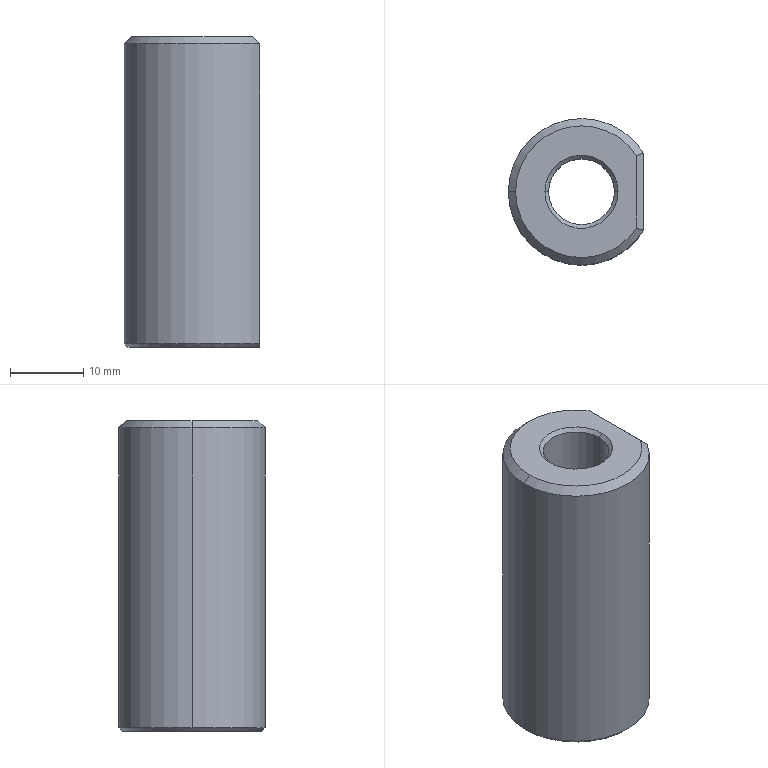Part | STEP file | Limit sleeve | 1 solid | 19 faces | box 18.5 x 20 x 42.5 mm | volume 8069 mm3 | cone 9 | cylinder 6 | plane 4 | commonest cylinder face diameters 9 x2 15 x2 20 x2
STEP:
#1=CARTESIAN_POINT('',(0.,0.,0.));
#2=DIRECTION('',(0.,0.,1.));
#3=DIRECTION('',(1.,0.,0.));
#4=AXIS2_PLACEMENT_3D('',#1,#2,#3);
#5=CARTESIAN_POINT('',(8.5,-5.268,41.5));
#6=VERTEX_POINT('',#5);
#7=CARTESIAN_POINT('',(-10.,0.,41.5));
#8=VERTEX_POINT('',#7);
#9=CARTESIAN_POINT('',(0.,0.,41.5));
#10=DIRECTION('',(0.,0.,-1.));
#11=DIRECTION('',(-1.,0.,0.));
#12=AXIS2_PLACEMENT_3D('',#9,#10,#11);
#13=CIRCLE('',#12,10.);
#14=CARTESIAN_POINT('',(0.,0.,42.5));
#15=DIRECTION('',(0.,0.,-1.));
#16=DIRECTION('',(-1.,0.,0.));
#17=AXIS2_PLACEMENT_3D('',#14,#15,#16);
#18=CYLINDRICAL_SURFACE('',#17,10.);
#19=CARTESIAN_POINT('',(0.,1.));
#20=DIRECTION('',(1.,0.));
#21=VECTOR('',#20,1.);
#22=LINE('',#19,#21);
#23=(GEOMETRIC_REPRESENTATION_CONTEXT(2)PARAMETRIC_REPRESENTATION_CONTEXT()REPRESENTATION_CONTEXT('',''));
#24=DEFINITIONAL_REPRESENTATION('',(#22),#23);
#25=PCURVE('',#18,#24);
#26=CARTESIAN_POINT('',(0.,0.,41.5));
#27=DIRECTION('',(0.,0.,-1.));
#28=DIRECTION('',(-1.,0.,0.));
#29=AXIS2_PLACEMENT_3D('',#26,#27,#28);
#30=CONICAL_SURFACE('',#29,10.,0.7854);
#31=CARTESIAN_POINT('',(0.,0.));
#32=DIRECTION('',(1.,0.));
#33=VECTOR('',#32,1.);
#34=LINE('',#31,#33);
#35=(GEOMETRIC_REPRESENTATION_CONTEXT(2)PARAMETRIC_REPRESENTATION_CONTEXT()REPRESENTATION_CONTEXT('',''));
#36=DEFINITIONAL_REPRESENTATION('',(#34),#35);
#37=PCURVE('',#30,#36);
#38=SURFACE_CURVE('',#13,(#25,#37),.PCURVE_S1.);
#39=EDGE_CURVE('',#6,#8,#38,.T.);
#40=ORIENTED_EDGE('',*,*,#39,.T.);
#41=CARTESIAN_POINT('',(-10.,0.,0.5));
#42=VERTEX_POINT('',#41);
#43=CARTESIAN_POINT('',(-10.,0.,42.5));
#44=DIRECTION('',(0.,0.,-1.));
#45=VECTOR('',#44,1.);
#46=LINE('',#43,#45);
#47=CARTESIAN_POINT('',(6.283,0.));
#48=DIRECTION('',(0.,1.));
#49=VECTOR('',#48,1.);
#50=LINE('',#47,#49);
#51=(GEOMETRIC_REPRESENTATION_CONTEXT(2)PARAMETRIC_REPRESENTATION_CONTEXT()REPRESENTATION_CONTEXT('',''));
#52=DEFINITIONAL_REPRESENTATION('',(#50),#51);
#53=PCURVE('',#18,#52);
#54=CARTESIAN_POINT('',(0.,0.,42.5));
#55=DIRECTION('',(0.,0.,-1.));
#56=DIRECTION('',(-1.,0.,0.));
#57=AXIS2_PLACEMENT_3D('',#54,#55,#56);
#58=CYLINDRICAL_SURFACE('',#57,10.);
#59=CARTESIAN_POINT('',(0.,0.));
#60=DIRECTION('',(0.,1.));
#61=VECTOR('',#60,1.);
#62=LINE('',#59,#61);
#63=(GEOMETRIC_REPRESENTATION_CONTEXT(2)PARAMETRIC_REPRESENTATION_CONTEXT()REPRESENTATION_CONTEXT('',''));
#64=DEFINITIONAL_REPRESENTATION('',(#62),#63);
#65=PCURVE('',#58,#64);
#66=SURFACE_CURVE('',#46,(#53,#65),.PCURVE_S1.);
#67=EDGE_CURVE('',#8,#42,#66,.T.);
#68=ORIENTED_EDGE('',*,*,#67,.T.);
#69=CARTESIAN_POINT('',(8.5,-5.268,0.5));
#70=VERTEX_POINT('',#69);
#71=CARTESIAN_POINT('',(0.,0.,0.5));
#72=DIRECTION('',(0.,0.,1.));
#73=DIRECTION('',(-1.,0.,0.));
#74=AXIS2_PLACEMENT_3D('',#71,#72,#73);
#75=CIRCLE('',#74,10.);
#76=CARTESIAN_POINT('',(6.283,42.));
#77=DIRECTION('',(-1.,0.));
#78=VECTOR('',#77,1.);
#79=LINE('',#76,#78);
#80=(GEOMETRIC_REPRESENTATION_CONTEXT(2)PARAMETRIC_REPRESENTATION_CONTEXT()REPRESENTATION_CONTEXT('',''));
#81=DEFINITIONAL_REPRESENTATION('',(#79),#80);
#82=PCURVE('',#18,#81);
#83=CARTESIAN_POINT('',(0.,0.,0.5));
#84=DIRECTION('',(0.,0.,1.));
#85=DIRECTION('',(1.,0.,0.));
#86=AXIS2_PLACEMENT_3D('',#83,#84,#85);
#87=CONICAL_SURFACE('',#86,10.,0.7854);
#88=CARTESIAN_POINT('',(3.142,0.));
#89=DIRECTION('',(1.,0.));
#90=VECTOR('',#89,1.);
#91=LINE('',#88,#90);
#92=(GEOMETRIC_REPRESENTATION_CONTEXT(2)PARAMETRIC_REPRESENTATION_CONTEXT()REPRESENTATION_CONTEXT('',''));
#93=DEFINITIONAL_REPRESENTATION('',(#91),#92);
#94=PCURVE('',#87,#93);
#95=SURFACE_CURVE('',#75,(#82,#94),.PCURVE_S1.);
#96=EDGE_CURVE('',#42,#70,#95,.T.);
#97=ORIENTED_EDGE('',*,*,#96,.T.);
#98=CARTESIAN_POINT('',(8.5,-5.268,42.5));
#99=DIRECTION('',(0.,0.,1.));
#100=VECTOR('',#99,1.);
#101=LINE('',#98,#100);
#102=CARTESIAN_POINT('',(3.696,0.));
#103=DIRECTION('',(0.,-1.));
#104=VECTOR('',#103,1.);
#105=LINE('',#102,#104);
#106=(GEOMETRIC_REPRESENTATION_CONTEXT(2)PARAMETRIC_REPRESENTATION_CONTEXT()REPRESENTATION_CONTEXT('',''));
#107=DEFINITIONAL_REPRESENTATION('',(#105),#106);
#108=PCURVE('',#18,#107);
#109=CARTESIAN_POINT('',(8.5,5.268,42.5));
#110=DIRECTION('',(-1.,0.,0.));
#111=DIRECTION('',(0.,0.,1.));
#112=AXIS2_PLACEMENT_3D('',#109,#110,#111);
#113=PLANE('',#112);
#114=CARTESIAN_POINT('',(0.,-10.536));
#115=DIRECTION('',(1.,0.));
#116=VECTOR('',#115,1.);
#117=LINE('',#114,#116);
#118=(GEOMETRIC_REPRESENTATION_CONTEXT(2)PARAMETRIC_REPRESENTATION_CONTEXT()REPRESENTATION_CONTEXT('',''));
#119=DEFINITIONAL_REPRESENTATION('',(#117),#118);
#120=PCURVE('',#113,#119);
#121=SURFACE_CURVE('',#101,(#108,#120),.PCURVE_S1.);
#122=EDGE_CURVE('',#70,#6,#121,.T.);
#123=ORIENTED_EDGE('',*,*,#122,.T.);
#124=EDGE_LOOP('',(#40,#68,#97,#123));
#125=FACE_BOUND('',#124,.T.);
#126=ADVANCED_FACE('',(#125),#18,.T.);
#127=CARTESIAN_POINT('',(7.5,-4.975,42.5));
#128=VERTEX_POINT('',#127);
#129=CARTESIAN_POINT('',(-9.,0.,42.5));
#130=VERTEX_POINT('',#129);
#131=CARTESIAN_POINT('',(0.,0.,42.5));
#132=DIRECTION('',(0.,0.,-1.));
#133=DIRECTION('',(-1.,0.,0.));
#134=AXIS2_PLACEMENT_3D('',#131,#132,#133);
#135=CIRCLE('',#134,9.);
#136=CARTESIAN_POINT('',(0.,-1.));
#137=DIRECTION('',(1.,0.));
#138=VECTOR('',#137,1.);
#139=LINE('',#136,#138);
#140=(GEOMETRIC_REPRESENTATION_CONTEXT(2)PARAMETRIC_REPRESENTATION_CONTEXT()REPRESENTATION_CONTEXT('',''));
#141=DEFINITIONAL_REPRESENTATION('',(#139),#140);
#142=PCURVE('',#30,#141);
#143=CARTESIAN_POINT('',(0.,0.,42.5));
#144=DIRECTION('',(0.,0.,1.));
#145=DIRECTION('',(1.,0.,0.));
#146=AXIS2_PLACEMENT_3D('',#143,#144,#145);
#147=PLANE('',#146);
#148=CARTESIAN_POINT('',(-9.,0.));
#149=CARTESIAN_POINT('',(-9.,15.588));
#150=CARTESIAN_POINT('',(4.5,7.794));
#151=CARTESIAN_POINT('',(18.,0.));
#152=CARTESIAN_POINT('',(4.5,-7.794));
#153=CARTESIAN_POINT('',(-9.,-15.588));
#154=CARTESIAN_POINT('',(-9.,0.));
#155=(BOUNDED_CURVE()B_SPLINE_CURVE(2,(#148,#149,#150,#151,#152,#153,#154),.UNSPECIFIED.,.T.,.F.)B_SPLINE_CURVE_WITH_KNOTS((1,2,2,2,2,1),(-2.094,0.,2.094,4.189,6.283,8.378),.UNSPECIFIED.)CURVE()GEOMETRIC_REPRESENTATION_ITEM()RATIONAL_B_SPLINE_CURVE((1.,0.5,1.,0.5,1.,0.5,1.))REPRESENTATION_ITEM(''));
#156=(GEOMETRIC_REPRESENTATION_CONTEXT(2)PARAMETRIC_REPRESENTATION_CONTEXT()REPRESENTATION_CONTEXT('',''));
#157=DEFINITIONAL_REPRESENTATION('',(#155),#156);
#158=PCURVE('',#147,#157);
#159=SURFACE_CURVE('',#135,(#142,#158),.PCURVE_S1.);
#160=EDGE_CURVE('',#128,#130,#159,.T.);
#161=ORIENTED_EDGE('',*,*,#160,.T.);
#162=CARTESIAN_POINT('',(-10.,0.,41.5));
#163=DIRECTION('',(-0.7071,0.,-0.7071));
#164=VECTOR('',#163,1.);
#165=LINE('',#162,#164);
#166=CARTESIAN_POINT('',(6.283,0.));
#167=DIRECTION('',(0.,1.));
#168=VECTOR('',#167,1.);
#169=LINE('',#166,#168);
#170=(GEOMETRIC_REPRESENTATION_CONTEXT(2)PARAMETRIC_REPRESENTATION_CONTEXT()REPRESENTATION_CONTEXT('',''));
#171=DEFINITIONAL_REPRESENTATION('',(#169),#170);
#172=PCURVE('',#30,#171);
#173=CARTESIAN_POINT('',(0.,0.,41.5));
#174=DIRECTION('',(0.,0.,-1.));
#175=DIRECTION('',(-1.,0.,0.));
#176=AXIS2_PLACEMENT_3D('',#173,#174,#175);
#177=CONICAL_SURFACE('',#176,10.,0.7854);
#178=CARTESIAN_POINT('',(0.,0.));
#179=DIRECTION('',(0.,1.));
#180=VECTOR('',#179,1.);
#181=LINE('',#178,#180);
#182=(GEOMETRIC_REPRESENTATION_CONTEXT(2)PARAMETRIC_REPRESENTATION_CONTEXT()REPRESENTATION_CONTEXT('',''));
#183=DEFINITIONAL_REPRESENTATION('',(#181),#182);
#184=PCURVE('',#177,#183);
#185=SURFACE_CURVE('',#165,(#172,#184),.PCURVE_S1.);
#186=EDGE_CURVE('',#130,#8,#185,.T.);
#187=ORIENTED_EDGE('',*,*,#186,.T.);
#188=ORIENTED_EDGE('',*,*,#39,.F.);
#189=CARTESIAN_POINT('',(8.5,-5.268,41.5));
#190=CARTESIAN_POINT('',(8.152,-5.169,41.848));
#191=CARTESIAN_POINT('',(7.818,-5.071,42.182));
#192=CARTESIAN_POINT('',(7.5,-4.975,42.5));
#193=B_SPLINE_CURVE_WITH_KNOTS('',3,(#189,#190,#191,#192),.UNSPECIFIED.,.F.,.F.,(4,4),(0.,1.),.PIECEWISE_BEZIER_KNOTS.);
#194=CARTESIAN_POINT('',(3.696,0.));
#195=CARTESIAN_POINT('',(3.697,-0.01584));
#196=CARTESIAN_POINT('',(3.698,-0.04744));
#197=CARTESIAN_POINT('',(3.699,-0.09467));
#198=CARTESIAN_POINT('',(3.7,-0.1417));
#199=CARTESIAN_POINT('',(3.702,-0.1886));
#200=CARTESIAN_POINT('',(3.703,-0.2352));
#201=CARTESIAN_POINT('',(3.705,-0.2817));
#202=CARTESIAN_POINT('',(3.706,-0.328));
#203=CARTESIAN_POINT('',(3.707,-0.3741));
#204=CARTESIAN_POINT('',(3.709,-0.42));
#205=CARTESIAN_POINT('',(3.71,-0.4658));
#206=CARTESIAN_POINT('',(3.712,-0.5113));
#207=CARTESIAN_POINT('',(3.713,-0.5567));
#208=CARTESIAN_POINT('',(3.714,-0.6019));
#209=CARTESIAN_POINT('',(3.716,-0.6468));
#210=CARTESIAN_POINT('',(3.717,-0.6916));
#211=CARTESIAN_POINT('',(3.719,-0.7363));
#212=CARTESIAN_POINT('',(3.72,-0.7807));
#213=CARTESIAN_POINT('',(3.721,-0.8249));
#214=CARTESIAN_POINT('',(3.723,-0.869));
#215=CARTESIAN_POINT('',(3.724,-0.9129));
#216=CARTESIAN_POINT('',(3.726,-0.9565));
#217=CARTESIAN_POINT('',(3.727,-0.9855));
#218=CARTESIAN_POINT('',(3.727,-1.));
#219=B_SPLINE_CURVE_WITH_KNOTS('',3,(#194,#195,#196,#197,#198,#199,#200,#201,#202,#203,#204,#205,#206,#207,#208,#209,#210,#211,#212,#213,#214,#215,#216,#217,#218),.UNSPECIFIED.,.F.,.F.,(4,1,1,1,1,1,1,1,1,1,1,1,1,1,1,1,1,1,1,1,1,1,4),(0.,0.04545,0.09091,0.1364,0.1818,0.2273,0.2727,0.3182,0.3636,0.4091,0.4545,0.5,0.5455,0.5909,0.6364,0.6818,0.7273,0.7727,0.8182,0.8636,0.9091,0.9545,1.),.QUASI_UNIFORM_KNOTS.);
#220=(GEOMETRIC_REPRESENTATION_CONTEXT(2)PARAMETRIC_REPRESENTATION_CONTEXT()REPRESENTATION_CONTEXT('',''));
#221=DEFINITIONAL_REPRESENTATION('',(#219),#220);
#222=PCURVE('',#30,#221);
#223=CARTESIAN_POINT('',(7.5,0.,42.5));
#224=DIRECTION('',(0.7071,0.,0.7071));
#225=DIRECTION('',(0.7071,0.,-0.7071));
#226=AXIS2_PLACEMENT_3D('',#223,#224,#225);
#227=PLANE('',#226);
#228=CARTESIAN_POINT('',(1.414,-5.268));
#229=CARTESIAN_POINT('',(0.9215,-5.169));
#230=CARTESIAN_POINT('',(0.4501,-5.071));
#231=CARTESIAN_POINT('',(0.,-4.975));
#232=B_SPLINE_CURVE_WITH_KNOTS('',3,(#228,#229,#230,#231),.UNSPECIFIED.,.F.,.F.,(4,4),(0.,1.),.PIECEWISE_BEZIER_KNOTS.);
#233=(GEOMETRIC_REPRESENTATION_CONTEXT(2)PARAMETRIC_REPRESENTATION_CONTEXT()REPRESENTATION_CONTEXT('',''));
#234=DEFINITIONAL_REPRESENTATION('',(#232),#233);
#235=PCURVE('',#227,#234);
#236=SURFACE_CURVE('',#193,(#222,#235),.PCURVE_S1.);
#237=EDGE_CURVE('',#6,#128,#236,.T.);
#238=ORIENTED_EDGE('',*,*,#237,.T.);
#239=EDGE_LOOP('',(#161,#187,#188,#238));
#240=FACE_BOUND('',#239,.T.);
#241=ADVANCED_FACE('',(#240),#30,.T.);
#242=CARTESIAN_POINT('',(-7.5,0.,0.5));
#243=VERTEX_POINT('',#242);
#244=CARTESIAN_POINT('',(-8.,0.,0.));
#245=VERTEX_POINT('',#244);
#246=CARTESIAN_POINT('',(-8.,0.,0.));
#247=DIRECTION('',(-0.7071,0.,-0.7071));
#248=VECTOR('',#247,1.);
#249=LINE('',#246,#248);
#250=CARTESIAN_POINT('',(0.,0.,0.));
#251=DIRECTION('',(0.,0.,-1.));
#252=DIRECTION('',(-1.,0.,0.));
#253=AXIS2_PLACEMENT_3D('',#250,#251,#252);
#254=CONICAL_SURFACE('',#253,8.,0.7854);
#255=CARTESIAN_POINT('',(6.283,0.));
#256=DIRECTION('',(0.,1.));
#257=VECTOR('',#256,1.);
#258=LINE('',#255,#257);
#259=(GEOMETRIC_REPRESENTATION_CONTEXT(2)PARAMETRIC_REPRESENTATION_CONTEXT()REPRESENTATION_CONTEXT('',''));
#260=DEFINITIONAL_REPRESENTATION('',(#258),#259);
#261=PCURVE('',#254,#260);
#262=CARTESIAN_POINT('',(0.,0.,0.));
#263=DIRECTION('',(0.,0.,-1.));
#264=DIRECTION('',(-1.,0.,0.));
#265=AXIS2_PLACEMENT_3D('',#262,#263,#264);
#266=CONICAL_SURFACE('',#265,8.,0.7854);
#267=CARTESIAN_POINT('',(0.,0.));
#268=DIRECTION('',(0.,1.));
#269=VECTOR('',#268,1.);
#270=LINE('',#267,#269);
#271=(GEOMETRIC_REPRESENTATION_CONTEXT(2)PARAMETRIC_REPRESENTATION_CONTEXT()REPRESENTATION_CONTEXT('',''));
#272=DEFINITIONAL_REPRESENTATION('',(#270),#271);
#273=PCURVE('',#266,#272);
#274=SURFACE_CURVE('',#249,(#261,#273),.PCURVE_S1.);
#275=EDGE_CURVE('',#243,#245,#274,.T.);
#276=ORIENTED_EDGE('',*,*,#275,.T.);
#277=CARTESIAN_POINT('',(8.,0.,0.));
#278=VERTEX_POINT('',#277);
#279=CARTESIAN_POINT('',(0.,0.,0.));
#280=DIRECTION('',(0.,0.,-1.));
#281=DIRECTION('',(-1.,0.,0.));
#282=AXIS2_PLACEMENT_3D('',#279,#280,#281);
#283=CIRCLE('',#282,8.);
#284=CARTESIAN_POINT('',(0.,0.));
#285=DIRECTION('',(1.,0.));
#286=VECTOR('',#285,1.);
#287=LINE('',#284,#286);
#288=(GEOMETRIC_REPRESENTATION_CONTEXT(2)PARAMETRIC_REPRESENTATION_CONTEXT()REPRESENTATION_CONTEXT('',''));
#289=DEFINITIONAL_REPRESENTATION('',(#287),#288);
#290=PCURVE('',#254,#289);
#291=CARTESIAN_POINT('',(0.,0.,0.));
#292=DIRECTION('',(0.,0.,1.));
#293=DIRECTION('',(1.,0.,0.));
#294=AXIS2_PLACEMENT_3D('',#291,#292,#293);
#295=PLANE('',#294);
#296=CARTESIAN_POINT('',(-8.,0.));
#297=CARTESIAN_POINT('',(-8.,13.856));
#298=CARTESIAN_POINT('',(4.,6.928));
#299=CARTESIAN_POINT('',(16.,0.));
#300=CARTESIAN_POINT('',(4.,-6.928));
#301=CARTESIAN_POINT('',(-8.,-13.856));
#302=CARTESIAN_POINT('',(-8.,0.));
#303=(BOUNDED_CURVE()B_SPLINE_CURVE(2,(#296,#297,#298,#299,#300,#301,#302),.UNSPECIFIED.,.T.,.F.)B_SPLINE_CURVE_WITH_KNOTS((1,2,2,2,2,1),(-2.094,0.,2.094,4.189,6.283,8.378),.UNSPECIFIED.)CURVE()GEOMETRIC_REPRESENTATION_ITEM()RATIONAL_B_SPLINE_CURVE((1.,0.5,1.,0.5,1.,0.5,1.))REPRESENTATION_ITEM(''));
#304=(GEOMETRIC_REPRESENTATION_CONTEXT(2)PARAMETRIC_REPRESENTATION_CONTEXT()REPRESENTATION_CONTEXT('',''));
#305=DEFINITIONAL_REPRESENTATION('',(#303),#304);
#306=PCURVE('',#295,#305);
#307=SURFACE_CURVE('',#283,(#290,#306),.PCURVE_S1.);
#308=EDGE_CURVE('',#278,#245,#307,.T.);
#309=ORIENTED_EDGE('',*,*,#308,.F.);
#310=CARTESIAN_POINT('',(7.5,0.,0.5));
#311=VERTEX_POINT('',#310);
#312=CARTESIAN_POINT('',(8.,0.,0.));
#313=DIRECTION('',(0.7071,0.,-0.7071));
#314=VECTOR('',#313,1.);
#315=LINE('',#312,#314);
#316=CARTESIAN_POINT('',(3.142,0.));
#317=DIRECTION('',(0.,1.));
#318=VECTOR('',#317,1.);
#319=LINE('',#316,#318);
#320=(GEOMETRIC_REPRESENTATION_CONTEXT(2)PARAMETRIC_REPRESENTATION_CONTEXT()REPRESENTATION_CONTEXT('',''));
#321=DEFINITIONAL_REPRESENTATION('',(#319),#320);
#322=PCURVE('',#254,#321);
#323=CARTESIAN_POINT('',(3.142,0.));
#324=DIRECTION('',(0.,1.));
#325=VECTOR('',#324,1.);
#326=LINE('',#323,#325);
#327=(GEOMETRIC_REPRESENTATION_CONTEXT(2)PARAMETRIC_REPRESENTATION_CONTEXT()REPRESENTATION_CONTEXT('',''));
#328=DEFINITIONAL_REPRESENTATION('',(#326),#327);
#329=PCURVE('',#266,#328);
#330=SURFACE_CURVE('',#315,(#322,#329),.PCURVE_S1.);
#331=EDGE_CURVE('',#311,#278,#330,.T.);
#332=ORIENTED_EDGE('',*,*,#331,.F.);
#333=CARTESIAN_POINT('',(0.,0.,0.5));
#334=DIRECTION('',(0.,0.,-1.));
#335=DIRECTION('',(-1.,0.,0.));
#336=AXIS2_PLACEMENT_3D('',#333,#334,#335);
#337=CIRCLE('',#336,7.5);
#338=CARTESIAN_POINT('',(0.,-0.5));
#339=DIRECTION('',(1.,0.));
#340=VECTOR('',#339,1.);
#341=LINE('',#338,#340);
#342=(GEOMETRIC_REPRESENTATION_CONTEXT(2)PARAMETRIC_REPRESENTATION_CONTEXT()REPRESENTATION_CONTEXT('',''));
#343=DEFINITIONAL_REPRESENTATION('',(#341),#342);
#344=PCURVE('',#254,#343);
#345=CARTESIAN_POINT('',(0.,0.,17.));
#346=DIRECTION('',(0.,0.,-1.));
#347=DIRECTION('',(-1.,0.,0.));
#348=AXIS2_PLACEMENT_3D('',#345,#346,#347);
#349=CYLINDRICAL_SURFACE('',#348,7.5);
#350=CARTESIAN_POINT('',(0.,16.5));
#351=DIRECTION('',(1.,0.));
#352=VECTOR('',#351,1.);
#353=LINE('',#350,#352);
#354=(GEOMETRIC_REPRESENTATION_CONTEXT(2)PARAMETRIC_REPRESENTATION_CONTEXT()REPRESENTATION_CONTEXT('',''));
#355=DEFINITIONAL_REPRESENTATION('',(#353),#354);
#356=PCURVE('',#349,#355);
#357=SURFACE_CURVE('',#337,(#344,#356),.PCURVE_S1.);
#358=EDGE_CURVE('',#311,#243,#357,.T.);
#359=ORIENTED_EDGE('',*,*,#358,.T.);
#360=EDGE_LOOP('',(#276,#309,#332,#359));
#361=FACE_BOUND('',#360,.F.);
#362=ADVANCED_FACE('',(#361),#254,.F.);
#363=CARTESIAN_POINT('',(4.5,0.,42.));
#364=VERTEX_POINT('',#363);
#365=CARTESIAN_POINT('',(5.,0.,42.5));
#366=VERTEX_POINT('',#365);
#367=CARTESIAN_POINT('',(5.,0.,42.5));
#368=DIRECTION('',(0.7071,0.,0.7071));
#369=VECTOR('',#368,1.);
#370=LINE('',#367,#369);
#371=CARTESIAN_POINT('',(0.,0.,42.5));
#372=DIRECTION('',(0.,0.,1.));
#373=DIRECTION('',(1.,0.,0.));
#374=AXIS2_PLACEMENT_3D('',#371,#372,#373);
#375=CONICAL_SURFACE('',#374,5.,0.7854);
#376=CARTESIAN_POINT('',(6.283,0.));
#377=DIRECTION('',(0.,1.));
#378=VECTOR('',#377,1.);
#379=LINE('',#376,#378);
#380=(GEOMETRIC_REPRESENTATION_CONTEXT(2)PARAMETRIC_REPRESENTATION_CONTEXT()REPRESENTATION_CONTEXT('',''));
#381=DEFINITIONAL_REPRESENTATION('',(#379),#380);
#382=PCURVE('',#375,#381);
#383=CARTESIAN_POINT('',(0.,0.,42.5));
#384=DIRECTION('',(0.,0.,1.));
#385=DIRECTION('',(1.,0.,0.));
#386=AXIS2_PLACEMENT_3D('',#383,#384,#385);
#387=CONICAL_SURFACE('',#386,5.,0.7854);
#388=CARTESIAN_POINT('',(0.,0.));
#389=DIRECTION('',(0.,1.));
#390=VECTOR('',#389,1.);
#391=LINE('',#388,#390);
#392=(GEOMETRIC_REPRESENTATION_CONTEXT(2)PARAMETRIC_REPRESENTATION_CONTEXT()REPRESENTATION_CONTEXT('',''));
#393=DEFINITIONAL_REPRESENTATION('',(#391),#392);
#394=PCURVE('',#387,#393);
#395=SURFACE_CURVE('',#370,(#382,#394),.PCURVE_S1.);
#396=EDGE_CURVE('',#364,#366,#395,.T.);
#397=ORIENTED_EDGE('',*,*,#396,.T.);
#398=CARTESIAN_POINT('',(-5.,0.,42.5));
#399=VERTEX_POINT('',#398);
#400=CARTESIAN_POINT('',(0.,0.,42.5));
#401=DIRECTION('',(0.,0.,-1.));
#402=DIRECTION('',(1.,0.,0.));
#403=AXIS2_PLACEMENT_3D('',#400,#401,#402);
#404=CIRCLE('',#403,5.);
#405=CARTESIAN_POINT('',(6.283,0.));
#406=DIRECTION('',(-1.,0.));
#407=VECTOR('',#406,1.);
#408=LINE('',#405,#407);
#409=(GEOMETRIC_REPRESENTATION_CONTEXT(2)PARAMETRIC_REPRESENTATION_CONTEXT()REPRESENTATION_CONTEXT('',''));
#410=DEFINITIONAL_REPRESENTATION('',(#408),#409);
#411=PCURVE('',#375,#410);
#412=CARTESIAN_POINT('',(5.,0.));
#413=CARTESIAN_POINT('',(5.,-8.66));
#414=CARTESIAN_POINT('',(-2.5,-4.33));
#415=CARTESIAN_POINT('',(-10.,0.));
#416=CARTESIAN_POINT('',(-2.5,4.33));
#417=CARTESIAN_POINT('',(5.,8.66));
#418=CARTESIAN_POINT('',(5.,0.));
#419=(BOUNDED_CURVE()B_SPLINE_CURVE(2,(#412,#413,#414,#415,#416,#417,#418),.UNSPECIFIED.,.T.,.F.)B_SPLINE_CURVE_WITH_KNOTS((1,2,2,2,2,1),(-2.094,0.,2.094,4.189,6.283,8.378),.UNSPECIFIED.)CURVE()GEOMETRIC_REPRESENTATION_ITEM()RATIONAL_B_SPLINE_CURVE((1.,0.5,1.,0.5,1.,0.5,1.))REPRESENTATION_ITEM(''));
#420=(GEOMETRIC_REPRESENTATION_CONTEXT(2)PARAMETRIC_REPRESENTATION_CONTEXT()REPRESENTATION_CONTEXT('',''));
#421=DEFINITIONAL_REPRESENTATION('',(#419),#420);
#422=PCURVE('',#147,#421);
#423=SURFACE_CURVE('',#404,(#411,#422),.PCURVE_S1.);
#424=EDGE_CURVE('',#366,#399,#423,.T.);
#425=ORIENTED_EDGE('',*,*,#424,.T.);
#426=CARTESIAN_POINT('',(-4.5,0.,42.));
#427=VERTEX_POINT('',#426);
#428=CARTESIAN_POINT('',(-5.,0.,42.5));
#429=DIRECTION('',(-0.7071,0.,0.7071));
#430=VECTOR('',#429,1.);
#431=LINE('',#428,#430);
#432=CARTESIAN_POINT('',(3.142,0.));
#433=DIRECTION('',(0.,1.));
#434=VECTOR('',#433,1.);
#435=LINE('',#432,#434);
#436=(GEOMETRIC_REPRESENTATION_CONTEXT(2)PARAMETRIC_REPRESENTATION_CONTEXT()REPRESENTATION_CONTEXT('',''));
#437=DEFINITIONAL_REPRESENTATION('',(#435),#436);
#438=PCURVE('',#375,#437);
#439=CARTESIAN_POINT('',(3.142,0.));
#440=DIRECTION('',(0.,1.));
#441=VECTOR('',#440,1.);
#442=LINE('',#439,#441);
#443=(GEOMETRIC_REPRESENTATION_CONTEXT(2)PARAMETRIC_REPRESENTATION_CONTEXT()REPRESENTATION_CONTEXT('',''));
#444=DEFINITIONAL_REPRESENTATION('',(#442),#443);
#445=PCURVE('',#387,#444);
#446=SURFACE_CURVE('',#431,(#438,#445),.PCURVE_S1.);
#447=EDGE_CURVE('',#427,#399,#446,.T.);
#448=ORIENTED_EDGE('',*,*,#447,.F.);
#449=CARTESIAN_POINT('',(0.,0.,42.));
#450=DIRECTION('',(0.,0.,1.));
#451=DIRECTION('',(1.,0.,0.));
#452=AXIS2_PLACEMENT_3D('',#449,#450,#451);
#453=CIRCLE('',#452,4.5);
#454=CARTESIAN_POINT('',(0.,-0.5));
#455=DIRECTION('',(1.,0.));
#456=VECTOR('',#455,1.);
#457=LINE('',#454,#456);
#458=(GEOMETRIC_REPRESENTATION_CONTEXT(2)PARAMETRIC_REPRESENTATION_CONTEXT()REPRESENTATION_CONTEXT('',''));
#459=DEFINITIONAL_REPRESENTATION('',(#457),#458);
#460=PCURVE('',#375,#459);
#461=CARTESIAN_POINT('',(0.,0.,0.));
#462=DIRECTION('',(0.,0.,1.));
#463=DIRECTION('',(1.,0.,0.));
#464=AXIS2_PLACEMENT_3D('',#461,#462,#463);
#465=CYLINDRICAL_SURFACE('',#464,4.5);
#466=CARTESIAN_POINT('',(0.,42.));
#467=DIRECTION('',(1.,0.));
#468=VECTOR('',#467,1.);
#469=LINE('',#466,#468);
#470=(GEOMETRIC_REPRESENTATION_CONTEXT(2)PARAMETRIC_REPRESENTATION_CONTEXT()REPRESENTATION_CONTEXT('',''));
#471=DEFINITIONAL_REPRESENTATION('',(#469),#470);
#472=PCURVE('',#465,#471);
#473=SURFACE_CURVE('',#453,(#460,#472),.PCURVE_S1.);
#474=EDGE_CURVE('',#427,#364,#473,.T.);
#475=ORIENTED_EDGE('',*,*,#474,.T.);
#476=EDGE_LOOP('',(#397,#425,#448,#475));
#477=FACE_BOUND('',#476,.F.);
#478=ADVANCED_FACE('',(#477),#375,.F.);
#479=CARTESIAN_POINT('',(-7.5,0.,17.));
#480=VERTEX_POINT('',#479);
#481=CARTESIAN_POINT('',(-7.5,0.,17.));
#482=DIRECTION('',(0.,0.,-1.));
#483=VECTOR('',#482,1.);
#484=LINE('',#481,#483);
#485=CARTESIAN_POINT('',(6.283,0.));
#486=DIRECTION('',(0.,1.));
#487=VECTOR('',#486,1.);
#488=LINE('',#485,#487);
#489=(GEOMETRIC_REPRESENTATION_CONTEXT(2)PARAMETRIC_REPRESENTATION_CONTEXT()REPRESENTATION_CONTEXT('',''));
#490=DEFINITIONAL_REPRESENTATION('',(#488),#489);
#491=PCURVE('',#349,#490);
#492=CARTESIAN_POINT('',(0.,0.,17.));
#493=DIRECTION('',(0.,0.,-1.));
#494=DIRECTION('',(-1.,0.,0.));
#495=AXIS2_PLACEMENT_3D('',#492,#493,#494);
#496=CYLINDRICAL_SURFACE('',#495,7.5);
#497=CARTESIAN_POINT('',(0.,0.));
#498=DIRECTION('',(0.,1.));
#499=VECTOR('',#498,1.);
#500=LINE('',#497,#499);
#501=(GEOMETRIC_REPRESENTATION_CONTEXT(2)PARAMETRIC_REPRESENTATION_CONTEXT()REPRESENTATION_CONTEXT('',''));
#502=DEFINITIONAL_REPRESENTATION('',(#500),#501);
#503=PCURVE('',#496,#502);
#504=SURFACE_CURVE('',#484,(#491,#503),.PCURVE_S1.);
#505=EDGE_CURVE('',#480,#243,#504,.T.);
#506=ORIENTED_EDGE('',*,*,#505,.T.);
#507=ORIENTED_EDGE('',*,*,#358,.F.);
#508=CARTESIAN_POINT('',(7.5,0.,17.));
#509=VERTEX_POINT('',#508);
#510=CARTESIAN_POINT('',(7.5,0.,17.));
#511=DIRECTION('',(0.,0.,-1.));
#512=VECTOR('',#511,1.);
#513=LINE('',#510,#512);
#514=CARTESIAN_POINT('',(3.142,0.));
#515=DIRECTION('',(0.,1.));
#516=VECTOR('',#515,1.);
#517=LINE('',#514,#516);
#518=(GEOMETRIC_REPRESENTATION_CONTEXT(2)PARAMETRIC_REPRESENTATION_CONTEXT()REPRESENTATION_CONTEXT('',''));
#519=DEFINITIONAL_REPRESENTATION('',(#517),#518);
#520=PCURVE('',#349,#519);
#521=CARTESIAN_POINT('',(3.142,0.));
#522=DIRECTION('',(0.,1.));
#523=VECTOR('',#522,1.);
#524=LINE('',#521,#523);
#525=(GEOMETRIC_REPRESENTATION_CONTEXT(2)PARAMETRIC_REPRESENTATION_CONTEXT()REPRESENTATION_CONTEXT('',''));
#526=DEFINITIONAL_REPRESENTATION('',(#524),#525);
#527=PCURVE('',#496,#526);
#528=SURFACE_CURVE('',#513,(#520,#527),.PCURVE_S1.);
#529=EDGE_CURVE('',#509,#311,#528,.T.);
#530=ORIENTED_EDGE('',*,*,#529,.F.);
#531=CARTESIAN_POINT('',(0.,0.,17.));
#532=DIRECTION('',(0.,0.,-1.));
#533=DIRECTION('',(-1.,0.,0.));
#534=AXIS2_PLACEMENT_3D('',#531,#532,#533);
#535=CIRCLE('',#534,7.5);
#536=CARTESIAN_POINT('',(0.,0.));
#537=DIRECTION('',(1.,0.));
#538=VECTOR('',#537,1.);
#539=LINE('',#536,#538);
#540=(GEOMETRIC_REPRESENTATION_CONTEXT(2)PARAMETRIC_REPRESENTATION_CONTEXT()REPRESENTATION_CONTEXT('',''));
#541=DEFINITIONAL_REPRESENTATION('',(#539),#540);
#542=PCURVE('',#349,#541);
#543=CARTESIAN_POINT('',(0.,0.,17.));
#544=DIRECTION('',(0.,0.,-1.));
#545=DIRECTION('',(-1.,0.,0.));
#546=AXIS2_PLACEMENT_3D('',#543,#544,#545);
#547=CONICAL_SURFACE('',#546,7.5,0.7854);
#548=CARTESIAN_POINT('',(0.,0.));
#549=DIRECTION('',(1.,0.));
#550=VECTOR('',#549,1.);
#551=LINE('',#548,#550);
#552=(GEOMETRIC_REPRESENTATION_CONTEXT(2)PARAMETRIC_REPRESENTATION_CONTEXT()REPRESENTATION_CONTEXT('',''));
#553=DEFINITIONAL_REPRESENTATION('',(#551),#552);
#554=PCURVE('',#547,#553);
#555=SURFACE_CURVE('',#535,(#542,#554),.PCURVE_S1.);
#556=EDGE_CURVE('',#509,#480,#555,.T.);
#557=ORIENTED_EDGE('',*,*,#556,.T.);
#558=EDGE_LOOP('',(#506,#507,#530,#557));
#559=FACE_BOUND('',#558,.F.);
#560=ADVANCED_FACE('',(#559),#349,.F.);
#561=CARTESIAN_POINT('',(4.5,0.,20.));
#562=VERTEX_POINT('',#561);
#563=CARTESIAN_POINT('',(4.5,0.,0.));
#564=DIRECTION('',(0.,0.,1.));
#565=VECTOR('',#564,1.);
#566=LINE('',#563,#565);
#567=CARTESIAN_POINT('',(6.283,0.));
#568=DIRECTION('',(0.,1.));
#569=VECTOR('',#568,1.);
#570=LINE('',#567,#569);
#571=(GEOMETRIC_REPRESENTATION_CONTEXT(2)PARAMETRIC_REPRESENTATION_CONTEXT()REPRESENTATION_CONTEXT('',''));
#572=DEFINITIONAL_REPRESENTATION('',(#570),#571);
#573=PCURVE('',#465,#572);
#574=CARTESIAN_POINT('',(0.,0.,0.));
#575=DIRECTION('',(0.,0.,1.));
#576=DIRECTION('',(1.,0.,0.));
#577=AXIS2_PLACEMENT_3D('',#574,#575,#576);
#578=CYLINDRICAL_SURFACE('',#577,4.5);
#579=CARTESIAN_POINT('',(0.,0.));
#580=DIRECTION('',(0.,1.));
#581=VECTOR('',#580,1.);
#582=LINE('',#579,#581);
#583=(GEOMETRIC_REPRESENTATION_CONTEXT(2)PARAMETRIC_REPRESENTATION_CONTEXT()REPRESENTATION_CONTEXT('',''));
#584=DEFINITIONAL_REPRESENTATION('',(#582),#583);
#585=PCURVE('',#578,#584);
#586=SURFACE_CURVE('',#566,(#573,#585),.PCURVE_S1.);
#587=EDGE_CURVE('',#562,#364,#586,.T.);
#588=ORIENTED_EDGE('',*,*,#587,.T.);
#589=ORIENTED_EDGE('',*,*,#474,.F.);
#590=CARTESIAN_POINT('',(-4.5,0.,20.));
#591=VERTEX_POINT('',#590);
#592=CARTESIAN_POINT('',(-4.5,0.,0.));
#593=DIRECTION('',(0.,0.,1.));
#594=VECTOR('',#593,1.);
#595=LINE('',#592,#594);
#596=CARTESIAN_POINT('',(3.142,0.));
#597=DIRECTION('',(0.,1.));
#598=VECTOR('',#597,1.);
#599=LINE('',#596,#598);
#600=(GEOMETRIC_REPRESENTATION_CONTEXT(2)PARAMETRIC_REPRESENTATION_CONTEXT()REPRESENTATION_CONTEXT('',''));
#601=DEFINITIONAL_REPRESENTATION('',(#599),#600);
#602=PCURVE('',#465,#601);
#603=CARTESIAN_POINT('',(3.142,0.));
#604=DIRECTION('',(0.,1.));
#605=VECTOR('',#604,1.);
#606=LINE('',#603,#605);
#607=(GEOMETRIC_REPRESENTATION_CONTEXT(2)PARAMETRIC_REPRESENTATION_CONTEXT()REPRESENTATION_CONTEXT('',''));
#608=DEFINITIONAL_REPRESENTATION('',(#606),#607);
#609=PCURVE('',#578,#608);
#610=SURFACE_CURVE('',#595,(#602,#609),.PCURVE_S1.);
#611=EDGE_CURVE('',#591,#427,#610,.T.);
#612=ORIENTED_EDGE('',*,*,#611,.F.);
#613=CARTESIAN_POINT('',(0.,0.,20.));
#614=DIRECTION('',(0.,0.,1.));
#615=DIRECTION('',(1.,0.,0.));
#616=AXIS2_PLACEMENT_3D('',#613,#614,#615);
#617=CIRCLE('',#616,4.5);
#618=CARTESIAN_POINT('',(0.,20.));
#619=DIRECTION('',(1.,0.));
#620=VECTOR('',#619,1.);
#621=LINE('',#618,#620);
#622=(GEOMETRIC_REPRESENTATION_CONTEXT(2)PARAMETRIC_REPRESENTATION_CONTEXT()REPRESENTATION_CONTEXT('',''));
#623=DEFINITIONAL_REPRESENTATION('',(#621),#622);
#624=PCURVE('',#465,#623);
#625=CARTESIAN_POINT('',(9.425,-3.));
#626=DIRECTION('',(-1.,0.));
#627=VECTOR('',#626,1.);
#628=LINE('',#625,#627);
#629=(GEOMETRIC_REPRESENTATION_CONTEXT(2)PARAMETRIC_REPRESENTATION_CONTEXT()REPRESENTATION_CONTEXT('',''));
#630=DEFINITIONAL_REPRESENTATION('',(#628),#629);
#631=PCURVE('',#547,#630);
#632=SURFACE_CURVE('',#617,(#624,#631),.PCURVE_S1.);
#633=EDGE_CURVE('',#591,#562,#632,.T.);
#634=ORIENTED_EDGE('',*,*,#633,.T.);
#635=EDGE_LOOP('',(#588,#589,#612,#634));
#636=FACE_BOUND('',#635,.F.);
#637=ADVANCED_FACE('',(#636),#465,.F.);
#638=CARTESIAN_POINT('',(-7.5,0.,17.));
#639=DIRECTION('',(-0.7071,0.,-0.7071));
#640=VECTOR('',#639,1.);
#641=LINE('',#638,#640);
#642=CARTESIAN_POINT('',(6.283,0.));
#643=DIRECTION('',(0.,1.));
#644=VECTOR('',#643,1.);
#645=LINE('',#642,#644);
#646=(GEOMETRIC_REPRESENTATION_CONTEXT(2)PARAMETRIC_REPRESENTATION_CONTEXT()REPRESENTATION_CONTEXT('',''));
#647=DEFINITIONAL_REPRESENTATION('',(#645),#646);
#648=PCURVE('',#547,#647);
#649=CARTESIAN_POINT('',(0.,0.,17.));
#650=DIRECTION('',(0.,0.,-1.));
#651=DIRECTION('',(-1.,0.,0.));
#652=AXIS2_PLACEMENT_3D('',#649,#650,#651);
#653=CONICAL_SURFACE('',#652,7.5,0.7854);
#654=CARTESIAN_POINT('',(0.,0.));
#655=DIRECTION('',(0.,1.));
#656=VECTOR('',#655,1.);
#657=LINE('',#654,#656);
#658=(GEOMETRIC_REPRESENTATION_CONTEXT(2)PARAMETRIC_REPRESENTATION_CONTEXT()REPRESENTATION_CONTEXT('',''));
#659=DEFINITIONAL_REPRESENTATION('',(#657),#658);
#660=PCURVE('',#653,#659);
#661=SURFACE_CURVE('',#641,(#648,#660),.PCURVE_S1.);
#662=EDGE_CURVE('',#591,#480,#661,.T.);
#663=ORIENTED_EDGE('',*,*,#662,.T.);
#664=ORIENTED_EDGE('',*,*,#556,.F.);
#665=CARTESIAN_POINT('',(7.5,0.,17.));
#666=DIRECTION('',(0.7071,0.,-0.7071));
#667=VECTOR('',#666,1.);
#668=LINE('',#665,#667);
#669=CARTESIAN_POINT('',(3.142,0.));
#670=DIRECTION('',(0.,1.));
#671=VECTOR('',#670,1.);
#672=LINE('',#669,#671);
#673=(GEOMETRIC_REPRESENTATION_CONTEXT(2)PARAMETRIC_REPRESENTATION_CONTEXT()REPRESENTATION_CONTEXT('',''));
#674=DEFINITIONAL_REPRESENTATION('',(#672),#673);
#675=PCURVE('',#547,#674);
#676=CARTESIAN_POINT('',(3.142,0.));
#677=DIRECTION('',(0.,1.));
#678=VECTOR('',#677,1.);
#679=LINE('',#676,#678);
#680=(GEOMETRIC_REPRESENTATION_CONTEXT(2)PARAMETRIC_REPRESENTATION_CONTEXT()REPRESENTATION_CONTEXT('',''));
#681=DEFINITIONAL_REPRESENTATION('',(#679),#680);
#682=PCURVE('',#653,#681);
#683=SURFACE_CURVE('',#668,(#675,#682),.PCURVE_S1.);
#684=EDGE_CURVE('',#562,#509,#683,.T.);
#685=ORIENTED_EDGE('',*,*,#684,.F.);
#686=ORIENTED_EDGE('',*,*,#633,.F.);
#687=EDGE_LOOP('',(#663,#664,#685,#686));
#688=FACE_BOUND('',#687,.F.);
#689=ADVANCED_FACE('',(#688),#547,.F.);
#690=ORIENTED_EDGE('',*,*,#67,.F.);
#691=CARTESIAN_POINT('',(8.5,5.268,41.5));
#692=VERTEX_POINT('',#691);
#693=CARTESIAN_POINT('',(0.,0.,41.5));
#694=DIRECTION('',(0.,0.,-1.));
#695=DIRECTION('',(-1.,0.,0.));
#696=AXIS2_PLACEMENT_3D('',#693,#694,#695);
#697=CIRCLE('',#696,10.);
#698=CARTESIAN_POINT('',(0.,1.));
#699=DIRECTION('',(1.,0.));
#700=VECTOR('',#699,1.);
#701=LINE('',#698,#700);
#702=(GEOMETRIC_REPRESENTATION_CONTEXT(2)PARAMETRIC_REPRESENTATION_CONTEXT()REPRESENTATION_CONTEXT('',''));
#703=DEFINITIONAL_REPRESENTATION('',(#701),#702);
#704=PCURVE('',#58,#703);
#705=CARTESIAN_POINT('',(0.,0.));
#706=DIRECTION('',(1.,0.));
#707=VECTOR('',#706,1.);
#708=LINE('',#705,#707);
#709=(GEOMETRIC_REPRESENTATION_CONTEXT(2)PARAMETRIC_REPRESENTATION_CONTEXT()REPRESENTATION_CONTEXT('',''));
#710=DEFINITIONAL_REPRESENTATION('',(#708),#709);
#711=PCURVE('',#177,#710);
#712=SURFACE_CURVE('',#697,(#704,#711),.PCURVE_S1.);
#713=EDGE_CURVE('',#8,#692,#712,.T.);
#714=ORIENTED_EDGE('',*,*,#713,.T.);
#715=CARTESIAN_POINT('',(8.5,5.268,0.5));
#716=VERTEX_POINT('',#715);
#717=CARTESIAN_POINT('',(8.5,5.268,42.5));
#718=DIRECTION('',(0.,0.,-1.));
#719=VECTOR('',#718,1.);
#720=LINE('',#717,#719);
#721=CARTESIAN_POINT('',(2.587,0.));
#722=DIRECTION('',(0.,1.));
#723=VECTOR('',#722,1.);
#724=LINE('',#721,#723);
#725=(GEOMETRIC_REPRESENTATION_CONTEXT(2)PARAMETRIC_REPRESENTATION_CONTEXT()REPRESENTATION_CONTEXT('',''));
#726=DEFINITIONAL_REPRESENTATION('',(#724),#725);
#727=PCURVE('',#58,#726);
#728=CARTESIAN_POINT('',(0.,0.));
#729=DIRECTION('',(-1.,0.));
#730=VECTOR('',#729,1.);
#731=LINE('',#728,#730);
#732=(GEOMETRIC_REPRESENTATION_CONTEXT(2)PARAMETRIC_REPRESENTATION_CONTEXT()REPRESENTATION_CONTEXT('',''));
#733=DEFINITIONAL_REPRESENTATION('',(#731),#732);
#734=PCURVE('',#113,#733);
#735=SURFACE_CURVE('',#720,(#727,#734),.PCURVE_S1.);
#736=EDGE_CURVE('',#692,#716,#735,.T.);
#737=ORIENTED_EDGE('',*,*,#736,.T.);
#738=CARTESIAN_POINT('',(0.,0.,0.5));
#739=DIRECTION('',(0.,0.,1.));
#740=DIRECTION('',(-1.,0.,0.));
#741=AXIS2_PLACEMENT_3D('',#738,#739,#740);
#742=CIRCLE('',#741,10.);
#743=CARTESIAN_POINT('',(6.283,42.));
#744=DIRECTION('',(-1.,0.));
#745=VECTOR('',#744,1.);
#746=LINE('',#743,#745);
#747=(GEOMETRIC_REPRESENTATION_CONTEXT(2)PARAMETRIC_REPRESENTATION_CONTEXT()REPRESENTATION_CONTEXT('',''));
#748=DEFINITIONAL_REPRESENTATION('',(#746),#747);
#749=PCURVE('',#58,#748);
#750=CARTESIAN_POINT('',(-3.142,0.));
#751=DIRECTION('',(1.,0.));
#752=VECTOR('',#751,1.);
#753=LINE('',#750,#752);
#754=(GEOMETRIC_REPRESENTATION_CONTEXT(2)PARAMETRIC_REPRESENTATION_CONTEXT()REPRESENTATION_CONTEXT('',''));
#755=DEFINITIONAL_REPRESENTATION('',(#753),#754);
#756=PCURVE('',#87,#755);
#757=SURFACE_CURVE('',#742,(#749,#756),.PCURVE_S1.);
#758=EDGE_CURVE('',#716,#42,#757,.T.);
#759=ORIENTED_EDGE('',*,*,#758,.T.);
#760=EDGE_LOOP('',(#690,#714,#737,#759));
#761=FACE_BOUND('',#760,.T.);
#762=ADVANCED_FACE('',(#761),#58,.T.);
#763=CARTESIAN_POINT('',(8.5,5.268,41.5));
#764=DIRECTION('',(0.,1.,0.));
#765=VECTOR('',#764,1.);
#766=LINE('',#763,#765);
#767=CARTESIAN_POINT('',(-1.,0.));
#768=DIRECTION('',(0.,1.));
#769=VECTOR('',#768,1.);
#770=LINE('',#767,#769);
#771=(GEOMETRIC_REPRESENTATION_CONTEXT(2)PARAMETRIC_REPRESENTATION_CONTEXT()REPRESENTATION_CONTEXT('',''));
#772=DEFINITIONAL_REPRESENTATION('',(#770),#771);
#773=PCURVE('',#113,#772);
#774=CARTESIAN_POINT('',(1.414,5.268));
#775=DIRECTION('',(0.,1.));
#776=VECTOR('',#775,1.);
#777=LINE('',#774,#776);
#778=(GEOMETRIC_REPRESENTATION_CONTEXT(2)PARAMETRIC_REPRESENTATION_CONTEXT()REPRESENTATION_CONTEXT('',''));
#779=DEFINITIONAL_REPRESENTATION('',(#777),#778);
#780=PCURVE('',#227,#779);
#781=SURFACE_CURVE('',#766,(#773,#780),.PCURVE_S1.);
#782=EDGE_CURVE('',#6,#692,#781,.T.);
#783=ORIENTED_EDGE('',*,*,#782,.F.);
#784=ORIENTED_EDGE('',*,*,#122,.F.);
#785=CARTESIAN_POINT('',(8.5,-4.243,0.));
#786=VERTEX_POINT('',#785);
#787=CARTESIAN_POINT('',(8.5,-4.243,0.));
#788=CARTESIAN_POINT('',(8.5,-4.59,0.1551));
#789=CARTESIAN_POINT('',(8.5,-4.931,0.3227));
#790=CARTESIAN_POINT('',(8.5,-5.268,0.5));
#791=B_SPLINE_CURVE_WITH_KNOTS('',3,(#787,#788,#789,#790),.UNSPECIFIED.,.F.,.F.,(4,4),(0.,0.001141),.PIECEWISE_BEZIER_KNOTS.);
#792=CARTESIAN_POINT('',(-42.5,-9.51));
#793=CARTESIAN_POINT('',(-42.345,-9.858));
#794=CARTESIAN_POINT('',(-42.177,-10.199));
#795=CARTESIAN_POINT('',(-42.,-10.536));
#796=B_SPLINE_CURVE_WITH_KNOTS('',3,(#792,#793,#794,#795),.UNSPECIFIED.,.F.,.F.,(4,4),(0.,0.001141),.PIECEWISE_BEZIER_KNOTS.);
#797=(GEOMETRIC_REPRESENTATION_CONTEXT(2)PARAMETRIC_REPRESENTATION_CONTEXT()REPRESENTATION_CONTEXT('',''));
#798=DEFINITIONAL_REPRESENTATION('',(#796),#797);
#799=PCURVE('',#113,#798);
#800=CARTESIAN_POINT('',(5.82,-0.5));
#801=CARTESIAN_POINT('',(5.819,-0.4929));
#802=CARTESIAN_POINT('',(5.816,-0.4788));
#803=CARTESIAN_POINT('',(5.811,-0.4574));
#804=CARTESIAN_POINT('',(5.807,-0.4359));
#805=CARTESIAN_POINT('',(5.803,-0.4142));
#806=CARTESIAN_POINT('',(5.798,-0.3924));
#807=CARTESIAN_POINT('',(5.794,-0.3704));
#808=CARTESIAN_POINT('',(5.79,-0.3482));
#809=CARTESIAN_POINT('',(5.785,-0.326));
#810=CARTESIAN_POINT('',(5.781,-0.3036));
#811=CARTESIAN_POINT('',(5.777,-0.281));
#812=CARTESIAN_POINT('',(5.773,-0.2583));
#813=CARTESIAN_POINT('',(5.769,-0.2355));
#814=CARTESIAN_POINT('',(5.764,-0.2125));
#815=CARTESIAN_POINT('',(5.76,-0.1894));
#816=CARTESIAN_POINT('',(5.756,-0.1662));
#817=CARTESIAN_POINT('',(5.752,-0.1428));
#818=CARTESIAN_POINT('',(5.748,-0.1194));
#819=CARTESIAN_POINT('',(5.744,-0.09574));
#820=CARTESIAN_POINT('',(5.74,-0.072));
#821=CARTESIAN_POINT('',(5.736,-0.04813));
#822=CARTESIAN_POINT('',(5.732,-0.02414));
#823=CARTESIAN_POINT('',(5.73,-0.008059));
#824=CARTESIAN_POINT('',(5.728,0.));
#825=B_SPLINE_CURVE_WITH_KNOTS('',3,(#800,#801,#802,#803,#804,#805,#806,#807,#808,#809,#810,#811,#812,#813,#814,#815,#816,#817,#818,#819,#820,#821,#822,#823,#824),.UNSPECIFIED.,.F.,.F.,(4,1,1,1,1,1,1,1,1,1,1,1,1,1,1,1,1,1,1,1,1,1,4),(0.,0.00005185,0.0001037,0.0001555,0.0002074,0.0002592,0.0003111,0.0003629,0.0004148,0.0004666,0.0005185,0.0005703,0.0006222,0.000674,0.0007258,0.0007777,0.0008295,0.0008814,0.0009332,0.0009851,0.001037,0.001089,0.001141),.QUASI_UNIFORM_KNOTS.);
#826=(GEOMETRIC_REPRESENTATION_CONTEXT(2)PARAMETRIC_REPRESENTATION_CONTEXT()REPRESENTATION_CONTEXT('',''));
#827=DEFINITIONAL_REPRESENTATION('',(#825),#826);
#828=PCURVE('',#87,#827);
#829=SURFACE_CURVE('',#791,(#799,#828),.PCURVE_S1.);
#830=EDGE_CURVE('',#786,#70,#829,.T.);
#831=ORIENTED_EDGE('',*,*,#830,.F.);
#832=CARTESIAN_POINT('',(8.5,4.243,0.));
#833=VERTEX_POINT('',#832);
#834=CARTESIAN_POINT('',(8.5,5.268,0.));
#835=DIRECTION('',(0.,-1.,0.));
#836=VECTOR('',#835,1.);
#837=LINE('',#834,#836);
#838=CARTESIAN_POINT('',(-42.5,0.));
#839=DIRECTION('',(0.,-1.));
#840=VECTOR('',#839,1.);
#841=LINE('',#838,#840);
#842=(GEOMETRIC_REPRESENTATION_CONTEXT(2)PARAMETRIC_REPRESENTATION_CONTEXT()REPRESENTATION_CONTEXT('',''));
#843=DEFINITIONAL_REPRESENTATION('',(#841),#842);
#844=PCURVE('',#113,#843);
#845=CARTESIAN_POINT('',(8.5,5.268));
#846=DIRECTION('',(0.,-1.));
#847=VECTOR('',#846,1.);
#848=LINE('',#845,#847);
#849=(GEOMETRIC_REPRESENTATION_CONTEXT(2)PARAMETRIC_REPRESENTATION_CONTEXT()REPRESENTATION_CONTEXT('',''));
#850=DEFINITIONAL_REPRESENTATION('',(#848),#849);
#851=PCURVE('',#295,#850);
#852=SURFACE_CURVE('',#837,(#844,#851),.PCURVE_S1.);
#853=EDGE_CURVE('',#833,#786,#852,.T.);
#854=ORIENTED_EDGE('',*,*,#853,.F.);
#855=CARTESIAN_POINT('',(8.5,5.268,0.5));
#856=CARTESIAN_POINT('',(8.5,4.931,0.3227));
#857=CARTESIAN_POINT('',(8.5,4.59,0.1551));
#858=CARTESIAN_POINT('',(8.5,4.243,0.));
#859=B_SPLINE_CURVE_WITH_KNOTS('',3,(#855,#856,#857,#858),.UNSPECIFIED.,.F.,.F.,(4,4),(0.,0.001141),.PIECEWISE_BEZIER_KNOTS.);
#860=CARTESIAN_POINT('',(-42.,0.));
#861=CARTESIAN_POINT('',(-42.177,-0.3365));
#862=CARTESIAN_POINT('',(-42.345,-0.6778));
#863=CARTESIAN_POINT('',(-42.5,-1.025));
#864=B_SPLINE_CURVE_WITH_KNOTS('',3,(#860,#861,#862,#863),.UNSPECIFIED.,.F.,.F.,(4,4),(0.,0.001141),.PIECEWISE_BEZIER_KNOTS.);
#865=(GEOMETRIC_REPRESENTATION_CONTEXT(2)PARAMETRIC_REPRESENTATION_CONTEXT()REPRESENTATION_CONTEXT('',''));
#866=DEFINITIONAL_REPRESENTATION('',(#864),#865);
#867=PCURVE('',#113,#866);
#868=CARTESIAN_POINT('',(0.5548,0.));
#869=CARTESIAN_POINT('',(0.5535,-0.008059));
#870=CARTESIAN_POINT('',(0.5509,-0.02414));
#871=CARTESIAN_POINT('',(0.547,-0.04813));
#872=CARTESIAN_POINT('',(0.543,-0.072));
#873=CARTESIAN_POINT('',(0.539,-0.09574));
#874=CARTESIAN_POINT('',(0.535,-0.1194));
#875=CARTESIAN_POINT('',(0.531,-0.1428));
#876=CARTESIAN_POINT('',(0.5269,-0.1662));
#877=CARTESIAN_POINT('',(0.5228,-0.1894));
#878=CARTESIAN_POINT('',(0.5187,-0.2125));
#879=CARTESIAN_POINT('',(0.5146,-0.2355));
#880=CARTESIAN_POINT('',(0.5104,-0.2583));
#881=CARTESIAN_POINT('',(0.5062,-0.281));
#882=CARTESIAN_POINT('',(0.502,-0.3036));
#883=CARTESIAN_POINT('',(0.4978,-0.326));
#884=CARTESIAN_POINT('',(0.4935,-0.3482));
#885=CARTESIAN_POINT('',(0.4892,-0.3704));
#886=CARTESIAN_POINT('',(0.4849,-0.3924));
#887=CARTESIAN_POINT('',(0.4806,-0.4142));
#888=CARTESIAN_POINT('',(0.4762,-0.4359));
#889=CARTESIAN_POINT('',(0.4718,-0.4574));
#890=CARTESIAN_POINT('',(0.4674,-0.4788));
#891=CARTESIAN_POINT('',(0.4644,-0.4929));
#892=CARTESIAN_POINT('',(0.463,-0.5));
#893=B_SPLINE_CURVE_WITH_KNOTS('',3,(#868,#869,#870,#871,#872,#873,#874,#875,#876,#877,#878,#879,#880,#881,#882,#883,#884,#885,#886,#887,#888,#889,#890,#891,#892),.UNSPECIFIED.,.F.,.F.,(4,1,1,1,1,1,1,1,1,1,1,1,1,1,1,1,1,1,1,1,1,1,4),(0.,0.00005185,0.0001037,0.0001555,0.0002074,0.0002592,0.0003111,0.0003629,0.0004148,0.0004666,0.0005185,0.0005703,0.0006222,0.000674,0.0007258,0.0007777,0.0008295,0.0008814,0.0009332,0.0009851,0.001037,0.001089,0.001141),.QUASI_UNIFORM_KNOTS.);
#894=(GEOMETRIC_REPRESENTATION_CONTEXT(2)PARAMETRIC_REPRESENTATION_CONTEXT()REPRESENTATION_CONTEXT('',''));
#895=DEFINITIONAL_REPRESENTATION('',(#893),#894);
#896=PCURVE('',#87,#895);
#897=SURFACE_CURVE('',#859,(#867,#896),.PCURVE_S1.);
#898=EDGE_CURVE('',#716,#833,#897,.T.);
#899=ORIENTED_EDGE('',*,*,#898,.F.);
#900=ORIENTED_EDGE('',*,*,#736,.F.);
#901=EDGE_LOOP('',(#783,#784,#831,#854,#899,#900));
#902=FACE_BOUND('',#901,.T.);
#903=ADVANCED_FACE('',(#902),#113,.F.);
#904=ORIENTED_EDGE('',*,*,#758,.F.);
#905=ORIENTED_EDGE('',*,*,#898,.T.);
#906=CARTESIAN_POINT('',(0.,0.,0.));
#907=DIRECTION('',(0.,0.,1.));
#908=DIRECTION('',(1.,0.,0.));
#909=AXIS2_PLACEMENT_3D('',#906,#907,#908);
#910=CIRCLE('',#909,9.5);
#911=CARTESIAN_POINT('',(0.,-0.5));
#912=DIRECTION('',(1.,0.));
#913=VECTOR('',#912,1.);
#914=LINE('',#911,#913);
#915=(GEOMETRIC_REPRESENTATION_CONTEXT(2)PARAMETRIC_REPRESENTATION_CONTEXT()REPRESENTATION_CONTEXT('',''));
#916=DEFINITIONAL_REPRESENTATION('',(#914),#915);
#917=PCURVE('',#87,#916);
#918=CARTESIAN_POINT('',(0.,0.));
#919=DIRECTION('',(1.,0.));
#920=AXIS2_PLACEMENT_2D('',#918,#919);
#921=CIRCLE('',#920,9.5);
#922=(GEOMETRIC_REPRESENTATION_CONTEXT(2)PARAMETRIC_REPRESENTATION_CONTEXT()REPRESENTATION_CONTEXT('',''));
#923=DEFINITIONAL_REPRESENTATION('',(#921),#922);
#924=PCURVE('',#295,#923);
#925=SURFACE_CURVE('',#910,(#917,#924),.PCURVE_S1.);
#926=EDGE_CURVE('',#833,#786,#925,.T.);
#927=ORIENTED_EDGE('',*,*,#926,.T.);
#928=ORIENTED_EDGE('',*,*,#830,.T.);
#929=ORIENTED_EDGE('',*,*,#96,.F.);
#930=EDGE_LOOP('',(#904,#905,#927,#928,#929));
#931=FACE_BOUND('',#930,.T.);
#932=ADVANCED_FACE('',(#931),#87,.T.);
#933=ORIENTED_EDGE('',*,*,#186,.F.);
#934=CARTESIAN_POINT('',(7.5,4.975,42.5));
#935=VERTEX_POINT('',#934);
#936=CARTESIAN_POINT('',(0.,0.,42.5));
#937=DIRECTION('',(0.,0.,-1.));
#938=DIRECTION('',(-1.,0.,0.));
#939=AXIS2_PLACEMENT_3D('',#936,#937,#938);
#940=CIRCLE('',#939,9.);
#941=CARTESIAN_POINT('',(0.,-1.));
#942=DIRECTION('',(1.,0.));
#943=VECTOR('',#942,1.);
#944=LINE('',#941,#943);
#945=(GEOMETRIC_REPRESENTATION_CONTEXT(2)PARAMETRIC_REPRESENTATION_CONTEXT()REPRESENTATION_CONTEXT('',''));
#946=DEFINITIONAL_REPRESENTATION('',(#944),#945);
#947=PCURVE('',#177,#946);
#948=CARTESIAN_POINT('',(-9.,0.));
#949=CARTESIAN_POINT('',(-9.,15.588));
#950=CARTESIAN_POINT('',(4.5,7.794));
#951=CARTESIAN_POINT('',(18.,0.));
#952=CARTESIAN_POINT('',(4.5,-7.794));
#953=CARTESIAN_POINT('',(-9.,-15.588));
#954=CARTESIAN_POINT('',(-9.,0.));
#955=(BOUNDED_CURVE()B_SPLINE_CURVE(2,(#948,#949,#950,#951,#952,#953,#954),.UNSPECIFIED.,.T.,.F.)B_SPLINE_CURVE_WITH_KNOTS((1,2,2,2,2,1),(-2.094,0.,2.094,4.189,6.283,8.378),.UNSPECIFIED.)CURVE()GEOMETRIC_REPRESENTATION_ITEM()RATIONAL_B_SPLINE_CURVE((1.,0.5,1.,0.5,1.,0.5,1.))REPRESENTATION_ITEM(''));
#956=(GEOMETRIC_REPRESENTATION_CONTEXT(2)PARAMETRIC_REPRESENTATION_CONTEXT()REPRESENTATION_CONTEXT('',''));
#957=DEFINITIONAL_REPRESENTATION('',(#955),#956);
#958=PCURVE('',#147,#957);
#959=SURFACE_CURVE('',#940,(#947,#958),.PCURVE_S1.);
#960=EDGE_CURVE('',#130,#935,#959,.T.);
#961=ORIENTED_EDGE('',*,*,#960,.T.);
#962=CARTESIAN_POINT('',(8.5,5.268,41.5));
#963=CARTESIAN_POINT('',(8.157,5.17,41.843));
#964=CARTESIAN_POINT('',(7.824,5.073,42.176));
#965=CARTESIAN_POINT('',(7.5,4.975,42.5));
#966=B_SPLINE_CURVE_WITH_KNOTS('',3,(#962,#963,#964,#965),.UNSPECIFIED.,.F.,.F.,(4,4),(0.,1.),.PIECEWISE_BEZIER_KNOTS.);
#967=CARTESIAN_POINT('',(2.587,0.));
#968=CARTESIAN_POINT('',(2.586,-0.01558));
#969=CARTESIAN_POINT('',(2.585,-0.04671));
#970=CARTESIAN_POINT('',(2.584,-0.09329));
#971=CARTESIAN_POINT('',(2.583,-0.1398));
#972=CARTESIAN_POINT('',(2.581,-0.1861));
#973=CARTESIAN_POINT('',(2.58,-0.2323));
#974=CARTESIAN_POINT('',(2.579,-0.2784));
#975=CARTESIAN_POINT('',(2.577,-0.3244));
#976=CARTESIAN_POINT('',(2.576,-0.3703));
#977=CARTESIAN_POINT('',(2.575,-0.416));
#978=CARTESIAN_POINT('',(2.573,-0.4617));
#979=CARTESIAN_POINT('',(2.572,-0.5072));
#980=CARTESIAN_POINT('',(2.57,-0.5526));
#981=CARTESIAN_POINT('',(2.569,-0.5978));
#982=CARTESIAN_POINT('',(2.568,-0.643));
#983=CARTESIAN_POINT('',(2.566,-0.688));
#984=CARTESIAN_POINT('',(2.565,-0.733));
#985=CARTESIAN_POINT('',(2.563,-0.7778));
#986=CARTESIAN_POINT('',(2.562,-0.8225));
#987=CARTESIAN_POINT('',(2.56,-0.867));
#988=CARTESIAN_POINT('',(2.559,-0.9115));
#989=CARTESIAN_POINT('',(2.557,-0.9558));
#990=CARTESIAN_POINT('',(2.556,-0.9853));
#991=CARTESIAN_POINT('',(2.556,-1.));
#992=B_SPLINE_CURVE_WITH_KNOTS('',3,(#967,#968,#969,#970,#971,#972,#973,#974,#975,#976,#977,#978,#979,#980,#981,#982,#983,#984,#985,#986,#987,#988,#989,#990,#991),.UNSPECIFIED.,.F.,.F.,(4,1,1,1,1,1,1,1,1,1,1,1,1,1,1,1,1,1,1,1,1,1,4),(0.,0.04545,0.09091,0.1364,0.1818,0.2273,0.2727,0.3182,0.3636,0.4091,0.4545,0.5,0.5455,0.5909,0.6364,0.6818,0.7273,0.7727,0.8182,0.8636,0.9091,0.9545,1.),.QUASI_UNIFORM_KNOTS.);
#993=(GEOMETRIC_REPRESENTATION_CONTEXT(2)PARAMETRIC_REPRESENTATION_CONTEXT()REPRESENTATION_CONTEXT('',''));
#994=DEFINITIONAL_REPRESENTATION('',(#992),#993);
#995=PCURVE('',#177,#994);
#996=CARTESIAN_POINT('',(1.414,5.268));
#997=CARTESIAN_POINT('',(0.9293,5.17));
#998=CARTESIAN_POINT('',(0.4579,5.073));
#999=CARTESIAN_POINT('',(0.,4.975));
#1000=B_SPLINE_CURVE_WITH_KNOTS('',3,(#996,#997,#998,#999),.UNSPECIFIED.,.F.,.F.,(4,4),(0.,1.),.PIECEWISE_BEZIER_KNOTS.);
#1001=(GEOMETRIC_REPRESENTATION_CONTEXT(2)PARAMETRIC_REPRESENTATION_CONTEXT()REPRESENTATION_CONTEXT('',''));
#1002=DEFINITIONAL_REPRESENTATION('',(#1000),#1001);
#1003=PCURVE('',#227,#1002);
#1004=SURFACE_CURVE('',#966,(#995,#1003),.PCURVE_S1.);
#1005=EDGE_CURVE('',#692,#935,#1004,.T.);
#1006=ORIENTED_EDGE('',*,*,#1005,.F.);
#1007=ORIENTED_EDGE('',*,*,#713,.F.);
#1008=EDGE_LOOP('',(#933,#961,#1006,#1007));
#1009=FACE_BOUND('',#1008,.T.);
#1010=ADVANCED_FACE('',(#1009),#177,.T.);
#1011=ORIENTED_EDGE('',*,*,#1005,.T.);
#1012=CARTESIAN_POINT('',(7.5,0.,42.5));
#1013=DIRECTION('',(0.,-1.,0.));
#1014=VECTOR('',#1013,1.);
#1015=LINE('',#1012,#1014);
#1016=CARTESIAN_POINT('',(0.,0.));
#1017=DIRECTION('',(0.,-1.));
#1018=VECTOR('',#1017,1.);
#1019=LINE('',#1016,#1018);
#1020=(GEOMETRIC_REPRESENTATION_CONTEXT(2)PARAMETRIC_REPRESENTATION_CONTEXT()REPRESENTATION_CONTEXT('',''));
#1021=DEFINITIONAL_REPRESENTATION('',(#1019),#1020);
#1022=PCURVE('',#227,#1021);
#1023=CARTESIAN_POINT('',(7.5,0.));
#1024=DIRECTION('',(0.,-1.));
#1025=VECTOR('',#1024,1.);
#1026=LINE('',#1023,#1025);
#1027=(GEOMETRIC_REPRESENTATION_CONTEXT(2)PARAMETRIC_REPRESENTATION_CONTEXT()REPRESENTATION_CONTEXT('',''));
#1028=DEFINITIONAL_REPRESENTATION('',(#1026),#1027);
#1029=PCURVE('',#147,#1028);
#1030=SURFACE_CURVE('',#1015,(#1022,#1029),.PCURVE_S1.);
#1031=EDGE_CURVE('',#935,#128,#1030,.T.);
#1032=ORIENTED_EDGE('',*,*,#1031,.T.);
#1033=ORIENTED_EDGE('',*,*,#237,.F.);
#1034=ORIENTED_EDGE('',*,*,#782,.T.);
#1035=EDGE_LOOP('',(#1011,#1032,#1033,#1034));
#1036=FACE_BOUND('',#1035,.T.);
#1037=ADVANCED_FACE('',(#1036),#227,.T.);
#1038=ORIENTED_EDGE('',*,*,#926,.F.);
#1039=ORIENTED_EDGE('',*,*,#853,.T.);
#1040=EDGE_LOOP('',(#1038,#1039));
#1041=FACE_BOUND('',#1040,.T.);
#1042=CARTESIAN_POINT('',(0.,0.,0.));
#1043=DIRECTION('',(0.,0.,-1.));
#1044=DIRECTION('',(-1.,0.,0.));
#1045=AXIS2_PLACEMENT_3D('',#1042,#1043,#1044);
#1046=CIRCLE('',#1045,8.);
#1047=CARTESIAN_POINT('',(-8.,0.));
#1048=CARTESIAN_POINT('',(-8.,13.856));
#1049=CARTESIAN_POINT('',(4.,6.928));
#1050=CARTESIAN_POINT('',(16.,0.));
#1051=CARTESIAN_POINT('',(4.,-6.928));
#1052=CARTESIAN_POINT('',(-8.,-13.856));
#1053=CARTESIAN_POINT('',(-8.,0.));
#1054=(BOUNDED_CURVE()B_SPLINE_CURVE(2,(#1047,#1048,#1049,#1050,#1051,#1052,#1053),.UNSPECIFIED.,.T.,.F.)B_SPLINE_CURVE_WITH_KNOTS((1,2,2,2,2,1),(-2.094,0.,2.094,4.189,6.283,8.378),.UNSPECIFIED.)CURVE()GEOMETRIC_REPRESENTATION_ITEM()RATIONAL_B_SPLINE_CURVE((1.,0.5,1.,0.5,1.,0.5,1.))REPRESENTATION_ITEM(''));
#1055=(GEOMETRIC_REPRESENTATION_CONTEXT(2)PARAMETRIC_REPRESENTATION_CONTEXT()REPRESENTATION_CONTEXT('',''));
#1056=DEFINITIONAL_REPRESENTATION('',(#1054),#1055);
#1057=PCURVE('',#295,#1056);
#1058=CARTESIAN_POINT('',(0.,0.));
#1059=DIRECTION('',(1.,0.));
#1060=VECTOR('',#1059,1.);
#1061=LINE('',#1058,#1060);
#1062=(GEOMETRIC_REPRESENTATION_CONTEXT(2)PARAMETRIC_REPRESENTATION_CONTEXT()REPRESENTATION_CONTEXT('',''));
#1063=DEFINITIONAL_REPRESENTATION('',(#1061),#1062);
#1064=PCURVE('',#266,#1063);
#1065=SURFACE_CURVE('',#1046,(#1057,#1064),.PCURVE_S1.);
#1066=EDGE_CURVE('',#245,#278,#1065,.T.);
#1067=ORIENTED_EDGE('',*,*,#1066,.F.);
#1068=ORIENTED_EDGE('',*,*,#308,.F.);
#1069=EDGE_LOOP('',(#1067,#1068));
#1070=FACE_BOUND('',#1069,.T.);
#1071=ADVANCED_FACE('',(#1041,#1070),#295,.F.);
#1072=ORIENTED_EDGE('',*,*,#424,.T.);
#1073=CARTESIAN_POINT('',(0.,0.,42.5));
#1074=DIRECTION('',(0.,0.,-1.));
#1075=DIRECTION('',(1.,0.,0.));
#1076=AXIS2_PLACEMENT_3D('',#1073,#1074,#1075);
#1077=CIRCLE('',#1076,5.);
#1078=CARTESIAN_POINT('',(5.,0.));
#1079=CARTESIAN_POINT('',(5.,-8.66));
#1080=CARTESIAN_POINT('',(-2.5,-4.33));
#1081=CARTESIAN_POINT('',(-10.,0.));
#1082=CARTESIAN_POINT('',(-2.5,4.33));
#1083=CARTESIAN_POINT('',(5.,8.66));
#1084=CARTESIAN_POINT('',(5.,0.));
#1085=(BOUNDED_CURVE()B_SPLINE_CURVE(2,(#1078,#1079,#1080,#1081,#1082,#1083,#1084),.UNSPECIFIED.,.T.,.F.)B_SPLINE_CURVE_WITH_KNOTS((1,2,2,2,2,1),(-2.094,0.,2.094,4.189,6.283,8.378),.UNSPECIFIED.)CURVE()GEOMETRIC_REPRESENTATION_ITEM()RATIONAL_B_SPLINE_CURVE((1.,0.5,1.,0.5,1.,0.5,1.))REPRESENTATION_ITEM(''));
#1086=(GEOMETRIC_REPRESENTATION_CONTEXT(2)PARAMETRIC_REPRESENTATION_CONTEXT()REPRESENTATION_CONTEXT('',''));
#1087=DEFINITIONAL_REPRESENTATION('',(#1085),#1086);
#1088=PCURVE('',#147,#1087);
#1089=CARTESIAN_POINT('',(6.283,0.));
#1090=DIRECTION('',(-1.,0.));
#1091=VECTOR('',#1090,1.);
#1092=LINE('',#1089,#1091);
#1093=(GEOMETRIC_REPRESENTATION_CONTEXT(2)PARAMETRIC_REPRESENTATION_CONTEXT()REPRESENTATION_CONTEXT('',''));
#1094=DEFINITIONAL_REPRESENTATION('',(#1092),#1093);
#1095=PCURVE('',#387,#1094);
#1096=SURFACE_CURVE('',#1077,(#1088,#1095),.PCURVE_S1.);
#1097=EDGE_CURVE('',#399,#366,#1096,.T.);
#1098=ORIENTED_EDGE('',*,*,#1097,.T.);
#1099=EDGE_LOOP('',(#1072,#1098));
#1100=FACE_BOUND('',#1099,.T.);
#1101=ORIENTED_EDGE('',*,*,#160,.F.);
#1102=ORIENTED_EDGE('',*,*,#1031,.F.);
#1103=ORIENTED_EDGE('',*,*,#960,.F.);
#1104=EDGE_LOOP('',(#1101,#1102,#1103));
#1105=FACE_BOUND('',#1104,.T.);
#1106=ADVANCED_FACE('',(#1100,#1105),#147,.T.);
#1107=ORIENTED_EDGE('',*,*,#1066,.F.);
#1108=ORIENTED_EDGE('',*,*,#275,.F.);
#1109=CARTESIAN_POINT('',(0.,0.,0.5));
#1110=DIRECTION('',(0.,0.,-1.));
#1111=DIRECTION('',(-1.,0.,0.));
#1112=AXIS2_PLACEMENT_3D('',#1109,#1110,#1111);
#1113=CIRCLE('',#1112,7.5);
#1114=CARTESIAN_POINT('',(0.,-0.5));
#1115=DIRECTION('',(1.,0.));
#1116=VECTOR('',#1115,1.);
#1117=LINE('',#1114,#1116);
#1118=(GEOMETRIC_REPRESENTATION_CONTEXT(2)PARAMETRIC_REPRESENTATION_CONTEXT()REPRESENTATION_CONTEXT('',''));
#1119=DEFINITIONAL_REPRESENTATION('',(#1117),#1118);
#1120=PCURVE('',#266,#1119);
#1121=CARTESIAN_POINT('',(0.,16.5));
#1122=DIRECTION('',(1.,0.));
#1123=VECTOR('',#1122,1.);
#1124=LINE('',#1121,#1123);
#1125=(GEOMETRIC_REPRESENTATION_CONTEXT(2)PARAMETRIC_REPRESENTATION_CONTEXT()REPRESENTATION_CONTEXT('',''));
#1126=DEFINITIONAL_REPRESENTATION('',(#1124),#1125);
#1127=PCURVE('',#496,#1126);
#1128=SURFACE_CURVE('',#1113,(#1120,#1127),.PCURVE_S1.);
#1129=EDGE_CURVE('',#243,#311,#1128,.T.);
#1130=ORIENTED_EDGE('',*,*,#1129,.T.);
#1131=ORIENTED_EDGE('',*,*,#331,.T.);
#1132=EDGE_LOOP('',(#1107,#1108,#1130,#1131));
#1133=FACE_BOUND('',#1132,.F.);
#1134=ADVANCED_FACE('',(#1133),#266,.F.);
#1135=ORIENTED_EDGE('',*,*,#1097,.T.);
#1136=ORIENTED_EDGE('',*,*,#396,.F.);
#1137=CARTESIAN_POINT('',(0.,0.,42.));
#1138=DIRECTION('',(0.,0.,1.));
#1139=DIRECTION('',(1.,0.,0.));
#1140=AXIS2_PLACEMENT_3D('',#1137,#1138,#1139);
#1141=CIRCLE('',#1140,4.5);
#1142=CARTESIAN_POINT('',(0.,-0.5));
#1143=DIRECTION('',(1.,0.));
#1144=VECTOR('',#1143,1.);
#1145=LINE('',#1142,#1144);
#1146=(GEOMETRIC_REPRESENTATION_CONTEXT(2)PARAMETRIC_REPRESENTATION_CONTEXT()REPRESENTATION_CONTEXT('',''));
#1147=DEFINITIONAL_REPRESENTATION('',(#1145),#1146);
#1148=PCURVE('',#387,#1147);
#1149=CARTESIAN_POINT('',(0.,42.));
#1150=DIRECTION('',(1.,0.));
#1151=VECTOR('',#1150,1.);
#1152=LINE('',#1149,#1151);
#1153=(GEOMETRIC_REPRESENTATION_CONTEXT(2)PARAMETRIC_REPRESENTATION_CONTEXT()REPRESENTATION_CONTEXT('',''));
#1154=DEFINITIONAL_REPRESENTATION('',(#1152),#1153);
#1155=PCURVE('',#578,#1154);
#1156=SURFACE_CURVE('',#1141,(#1148,#1155),.PCURVE_S1.);
#1157=EDGE_CURVE('',#364,#427,#1156,.T.);
#1158=ORIENTED_EDGE('',*,*,#1157,.T.);
#1159=ORIENTED_EDGE('',*,*,#447,.T.);
#1160=EDGE_LOOP('',(#1135,#1136,#1158,#1159));
#1161=FACE_BOUND('',#1160,.F.);
#1162=ADVANCED_FACE('',(#1161),#387,.F.);
#1163=ORIENTED_EDGE('',*,*,#1129,.F.);
#1164=ORIENTED_EDGE('',*,*,#505,.F.);
#1165=CARTESIAN_POINT('',(0.,0.,17.));
#1166=DIRECTION('',(0.,0.,-1.));
#1167=DIRECTION('',(-1.,0.,0.));
#1168=AXIS2_PLACEMENT_3D('',#1165,#1166,#1167);
#1169=CIRCLE('',#1168,7.5);
#1170=CARTESIAN_POINT('',(0.,0.));
#1171=DIRECTION('',(1.,0.));
#1172=VECTOR('',#1171,1.);
#1173=LINE('',#1170,#1172);
#1174=(GEOMETRIC_REPRESENTATION_CONTEXT(2)PARAMETRIC_REPRESENTATION_CONTEXT()REPRESENTATION_CONTEXT('',''));
#1175=DEFINITIONAL_REPRESENTATION('',(#1173),#1174);
#1176=PCURVE('',#496,#1175);
#1177=CARTESIAN_POINT('',(0.,0.));
#1178=DIRECTION('',(1.,0.));
#1179=VECTOR('',#1178,1.);
#1180=LINE('',#1177,#1179);
#1181=(GEOMETRIC_REPRESENTATION_CONTEXT(2)PARAMETRIC_REPRESENTATION_CONTEXT()REPRESENTATION_CONTEXT('',''));
#1182=DEFINITIONAL_REPRESENTATION('',(#1180),#1181);
#1183=PCURVE('',#653,#1182);
#1184=SURFACE_CURVE('',#1169,(#1176,#1183),.PCURVE_S1.);
#1185=EDGE_CURVE('',#480,#509,#1184,.T.);
#1186=ORIENTED_EDGE('',*,*,#1185,.T.);
#1187=ORIENTED_EDGE('',*,*,#529,.T.);
#1188=EDGE_LOOP('',(#1163,#1164,#1186,#1187));
#1189=FACE_BOUND('',#1188,.F.);
#1190=ADVANCED_FACE('',(#1189),#496,.F.);
#1191=ORIENTED_EDGE('',*,*,#1157,.F.);
#1192=ORIENTED_EDGE('',*,*,#587,.F.);
#1193=CARTESIAN_POINT('',(0.,0.,20.));
#1194=DIRECTION('',(0.,0.,1.));
#1195=DIRECTION('',(1.,0.,0.));
#1196=AXIS2_PLACEMENT_3D('',#1193,#1194,#1195);
#1197=CIRCLE('',#1196,4.5);
#1198=CARTESIAN_POINT('',(0.,20.));
#1199=DIRECTION('',(1.,0.));
#1200=VECTOR('',#1199,1.);
#1201=LINE('',#1198,#1200);
#1202=(GEOMETRIC_REPRESENTATION_CONTEXT(2)PARAMETRIC_REPRESENTATION_CONTEXT()REPRESENTATION_CONTEXT('',''));
#1203=DEFINITIONAL_REPRESENTATION('',(#1201),#1202);
#1204=PCURVE('',#578,#1203);
#1205=CARTESIAN_POINT('',(3.142,-3.));
#1206=DIRECTION('',(-1.,0.));
#1207=VECTOR('',#1206,1.);
#1208=LINE('',#1205,#1207);
#1209=(GEOMETRIC_REPRESENTATION_CONTEXT(2)PARAMETRIC_REPRESENTATION_CONTEXT()REPRESENTATION_CONTEXT('',''));
#1210=DEFINITIONAL_REPRESENTATION('',(#1208),#1209);
#1211=PCURVE('',#653,#1210);
#1212=SURFACE_CURVE('',#1197,(#1204,#1211),.PCURVE_S1.);
#1213=EDGE_CURVE('',#562,#591,#1212,.T.);
#1214=ORIENTED_EDGE('',*,*,#1213,.T.);
#1215=ORIENTED_EDGE('',*,*,#611,.T.);
#1216=EDGE_LOOP('',(#1191,#1192,#1214,#1215));
#1217=FACE_BOUND('',#1216,.F.);
#1218=ADVANCED_FACE('',(#1217),#578,.F.);
#1219=ORIENTED_EDGE('',*,*,#1185,.F.);
#1220=ORIENTED_EDGE('',*,*,#662,.F.);
#1221=ORIENTED_EDGE('',*,*,#1213,.F.);
#1222=ORIENTED_EDGE('',*,*,#684,.T.);
#1223=EDGE_LOOP('',(#1219,#1220,#1221,#1222));
#1224=FACE_BOUND('',#1223,.F.);
#1225=ADVANCED_FACE('',(#1224),#653,.F.);
#1226=CLOSED_SHELL('',(#126,#241,#362,#478,#560,#637,#689,#762,#903,#932,#1010,#1037,#1071,#1106,#1134,#1162,#1190,#1218,#1225));
#1227=MANIFOLD_SOLID_BREP('',#1226);
#1228=(LENGTH_UNIT()NAMED_UNIT(*)SI_UNIT(.MILLI.,.METRE.));
#1229=UNCERTAINTY_MEASURE_WITH_UNIT(LENGTH_MEASURE(0.000001),#1228,'','');
#1230=(NAMED_UNIT(*)PLANE_ANGLE_UNIT()SI_UNIT($,.RADIAN.));
#1231=(NAMED_UNIT(*)SI_UNIT($,.STERADIAN.)SOLID_ANGLE_UNIT());
#1232=(GEOMETRIC_REPRESENTATION_CONTEXT(3)GLOBAL_UNCERTAINTY_ASSIGNED_CONTEXT((#1229))GLOBAL_UNIT_ASSIGNED_CONTEXT((#1228,#1230,#1231))REPRESENTATION_CONTEXT('',''));
#1233=ADVANCED_BREP_SHAPE_REPRESENTATION('',(#4,#1227),#1232);